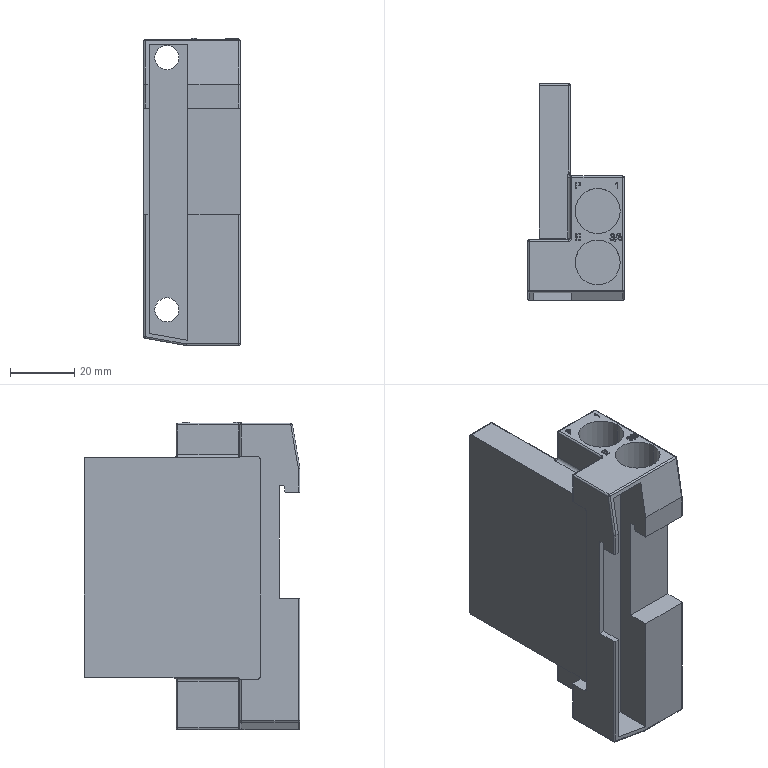Part | STEP file | SS5V1-16S3AD-08B-N1_CAInput Side End Plate | 1 solid | 196 faces | box 30 x 67.2 x 95.55 mm | volume 93320 mm3 | plane 91 | cylinder 51 | spline 32 | sphere 14 | torus 8 | commonest cylinder face diameters 1 x34 2 x5 2.5 x4 7.5 x4 14 x4